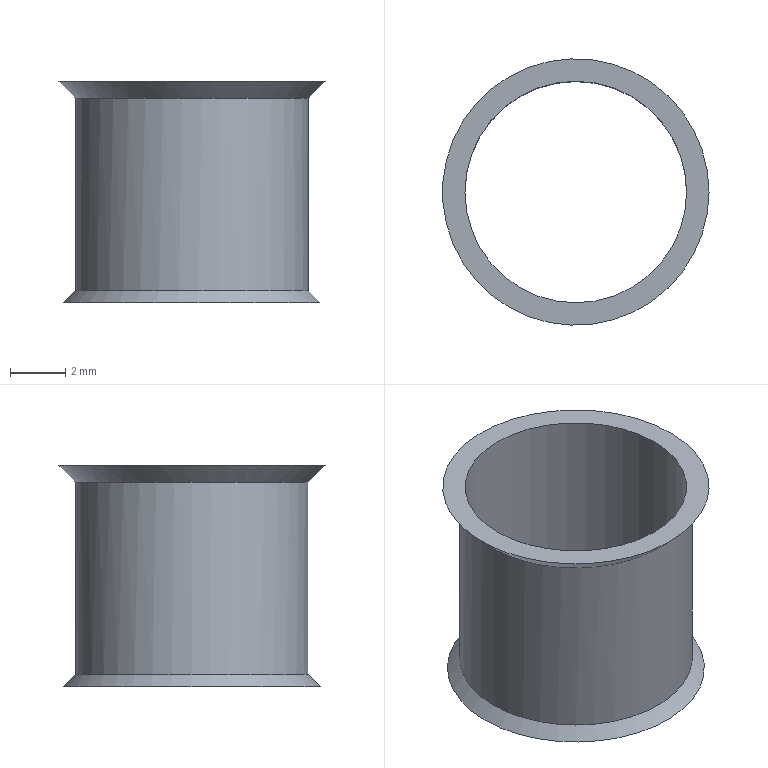Part | STEP file | 1 solid | 6 faces | box 9.62 x 9.62 x 8 mm | volume 49.009 mm3 | cylinder 2 | plane 2 | cone 2 | commonest cylinder face diameters 8 x1 8.4 x1
STEP:
#1=CARTESIAN_POINT('',(0.,0.,0.));
#2=DIRECTION('',(0.,0.,1.));
#3=DIRECTION('',(1.,0.,0.));
#4=AXIS2_PLACEMENT_3D('',#1,#2,#3);
#5=CARTESIAN_POINT('',(27.622,157.82,20.85));
#6=VERTEX_POINT('',#5);
#7=CARTESIAN_POINT('',(31.622,157.82,20.85));
#8=DIRECTION('',(0.,0.,1.));
#9=DIRECTION('',(-1.,0.,0.));
#10=AXIS2_PLACEMENT_3D('',#7,#8,#9);
#11=CIRCLE('',#10,4.);
#12=CARTESIAN_POINT('',(31.622,157.82,24.85));
#13=DIRECTION('',(0.,0.,-1.));
#14=DIRECTION('',(-1.,0.,0.));
#15=AXIS2_PLACEMENT_3D('',#12,#13,#14);
#16=CYLINDRICAL_SURFACE('',#15,4.);
#17=CARTESIAN_POINT('',(6.283,4.));
#18=DIRECTION('',(-1.,0.));
#19=VECTOR('',#18,1.);
#20=LINE('',#17,#19);
#21=(GEOMETRIC_REPRESENTATION_CONTEXT(2)PARAMETRIC_REPRESENTATION_CONTEXT()REPRESENTATION_CONTEXT('',''));
#22=DEFINITIONAL_REPRESENTATION('',(#20),#21);
#23=PCURVE('',#16,#22);
#24=CARTESIAN_POINT('',(39.122,157.82,20.85));
#25=DIRECTION('',(0.,0.,1.));
#26=DIRECTION('',(1.,0.,0.));
#27=AXIS2_PLACEMENT_3D('',#24,#25,#26);
#28=PLANE('',#27);
#29=CARTESIAN_POINT('',(-7.5,0.));
#30=DIRECTION('',(-1.,0.));
#31=AXIS2_PLACEMENT_2D('',#29,#30);
#32=CIRCLE('',#31,4.);
#33=(GEOMETRIC_REPRESENTATION_CONTEXT(2)PARAMETRIC_REPRESENTATION_CONTEXT()REPRESENTATION_CONTEXT('',''));
#34=DEFINITIONAL_REPRESENTATION('',(#32),#33);
#35=PCURVE('',#28,#34);
#36=SURFACE_CURVE('',#11,(#23,#35),.PCURVE_S1.);
#37=EDGE_CURVE('',#6,#6,#36,.T.);
#38=ORIENTED_EDGE('',*,*,#37,.T.);
#39=CARTESIAN_POINT('',(27.622,157.82,28.85));
#40=VERTEX_POINT('',#39);
#41=CARTESIAN_POINT('',(27.622,157.82,28.85));
#42=CARTESIAN_POINT('',(27.622,157.82,20.85));
#43=B_SPLINE_CURVE_WITH_KNOTS('',1,(#41,#42),.UNSPECIFIED.,.F.,.F.,(2,2),(-4.,4.),.PIECEWISE_BEZIER_KNOTS.);
#44=CARTESIAN_POINT('',(0.,0.));
#45=DIRECTION('',(0.,1.));
#46=VECTOR('',#45,1.);
#47=LINE('',#44,#46);
#48=(GEOMETRIC_REPRESENTATION_CONTEXT(2)PARAMETRIC_REPRESENTATION_CONTEXT()REPRESENTATION_CONTEXT('',''));
#49=DEFINITIONAL_REPRESENTATION('',(#47),#48);
#50=PCURVE('',#16,#49);
#51=CARTESIAN_POINT('',(6.283,0.));
#52=DIRECTION('',(0.,1.));
#53=VECTOR('',#52,1.);
#54=LINE('',#51,#53);
#55=(GEOMETRIC_REPRESENTATION_CONTEXT(2)PARAMETRIC_REPRESENTATION_CONTEXT()REPRESENTATION_CONTEXT('',''));
#56=DEFINITIONAL_REPRESENTATION('',(#54),#55);
#57=PCURVE('',#16,#56);
#58=SEAM_CURVE('',#43,(#50,#57),.PCURVE_S1.);
#59=EDGE_CURVE('',#40,#6,#58,.T.);
#60=ORIENTED_EDGE('',*,*,#59,.F.);
#61=CARTESIAN_POINT('',(31.622,157.82,28.85));
#62=DIRECTION('',(0.,0.,-1.));
#63=DIRECTION('',(-1.,0.,0.));
#64=AXIS2_PLACEMENT_3D('',#61,#62,#63);
#65=CIRCLE('',#64,4.);
#66=CARTESIAN_POINT('',(0.,-4.));
#67=DIRECTION('',(1.,0.));
#68=VECTOR('',#67,1.);
#69=LINE('',#66,#68);
#70=(GEOMETRIC_REPRESENTATION_CONTEXT(2)PARAMETRIC_REPRESENTATION_CONTEXT()REPRESENTATION_CONTEXT('',''));
#71=DEFINITIONAL_REPRESENTATION('',(#69),#70);
#72=PCURVE('',#16,#71);
#73=CARTESIAN_POINT('',(34.122,157.82,28.85));
#74=DIRECTION('',(0.,0.,-1.));
#75=DIRECTION('',(-1.,0.,0.));
#76=AXIS2_PLACEMENT_3D('',#73,#74,#75);
#77=PLANE('',#76);
#78=CARTESIAN_POINT('',(2.5,0.));
#79=DIRECTION('',(1.,0.));
#80=AXIS2_PLACEMENT_2D('',#78,#79);
#81=CIRCLE('',#80,4.);
#82=(GEOMETRIC_REPRESENTATION_CONTEXT(2)PARAMETRIC_REPRESENTATION_CONTEXT()REPRESENTATION_CONTEXT('',''));
#83=DEFINITIONAL_REPRESENTATION('',(#81),#82);
#84=PCURVE('',#77,#83);
#85=SURFACE_CURVE('',#65,(#72,#84),.PCURVE_S1.);
#86=EDGE_CURVE('',#40,#40,#85,.T.);
#87=ORIENTED_EDGE('',*,*,#86,.T.);
#88=ORIENTED_EDGE('',*,*,#59,.T.);
#89=EDGE_LOOP('',(#38,#60,#87,#88));
#90=FACE_BOUND('',#89,.F.);
#91=ADVANCED_FACE('',(#90),#16,.F.);
#92=ORIENTED_EDGE('',*,*,#86,.T.);
#93=EDGE_LOOP('',(#92));
#94=FACE_BOUND('',#93,.T.);
#95=CARTESIAN_POINT('',(36.432,157.82,28.85));
#96=VERTEX_POINT('',#95);
#97=CARTESIAN_POINT('',(31.622,157.82,28.85));
#98=DIRECTION('',(0.,0.,-1.));
#99=DIRECTION('',(1.,0.,0.));
#100=AXIS2_PLACEMENT_3D('',#97,#98,#99);
#101=CIRCLE('',#100,4.81);
#102=CARTESIAN_POINT('',(2.5,0.));
#103=DIRECTION('',(-1.,0.));
#104=AXIS2_PLACEMENT_2D('',#102,#103);
#105=CIRCLE('',#104,4.81);
#106=(GEOMETRIC_REPRESENTATION_CONTEXT(2)PARAMETRIC_REPRESENTATION_CONTEXT()REPRESENTATION_CONTEXT('',''));
#107=DEFINITIONAL_REPRESENTATION('',(#105),#106);
#108=PCURVE('',#77,#107);
#109=CARTESIAN_POINT('',(31.622,157.82,28.85));
#110=DIRECTION('',(0.,0.,1.));
#111=DIRECTION('',(1.,0.,0.));
#112=AXIS2_PLACEMENT_3D('',#109,#110,#111);
#113=CONICAL_SURFACE('',#112,4.81,0.7854);
#114=CARTESIAN_POINT('',(6.283,0.));
#115=DIRECTION('',(-1.,0.));
#116=VECTOR('',#115,1.);
#117=LINE('',#114,#116);
#118=(GEOMETRIC_REPRESENTATION_CONTEXT(2)PARAMETRIC_REPRESENTATION_CONTEXT()REPRESENTATION_CONTEXT('',''));
#119=DEFINITIONAL_REPRESENTATION('',(#117),#118);
#120=PCURVE('',#113,#119);
#121=SURFACE_CURVE('',#101,(#108,#120),.PCURVE_S1.);
#122=EDGE_CURVE('',#96,#96,#121,.T.);
#123=ORIENTED_EDGE('',*,*,#122,.F.);
#124=EDGE_LOOP('',(#123));
#125=FACE_BOUND('',#124,.T.);
#126=ADVANCED_FACE('',(#94,#125),#77,.F.);
#127=ORIENTED_EDGE('',*,*,#37,.T.);
#128=EDGE_LOOP('',(#127));
#129=FACE_BOUND('',#128,.T.);
#130=CARTESIAN_POINT('',(26.982,157.82,20.85));
#131=VERTEX_POINT('',#130);
#132=CARTESIAN_POINT('',(31.622,157.82,20.85));
#133=DIRECTION('',(0.,0.,1.));
#134=DIRECTION('',(-1.,0.,0.));
#135=AXIS2_PLACEMENT_3D('',#132,#133,#134);
#136=CIRCLE('',#135,4.64);
#137=CARTESIAN_POINT('',(-7.5,0.));
#138=DIRECTION('',(-1.,0.));
#139=AXIS2_PLACEMENT_2D('',#137,#138);
#140=CIRCLE('',#139,4.64);
#141=(GEOMETRIC_REPRESENTATION_CONTEXT(2)PARAMETRIC_REPRESENTATION_CONTEXT()REPRESENTATION_CONTEXT('',''));
#142=DEFINITIONAL_REPRESENTATION('',(#140),#141);
#143=PCURVE('',#28,#142);
#144=CARTESIAN_POINT('',(31.622,157.82,20.85));
#145=DIRECTION('',(0.,0.,-1.));
#146=DIRECTION('',(-1.,0.,0.));
#147=AXIS2_PLACEMENT_3D('',#144,#145,#146);
#148=CONICAL_SURFACE('',#147,4.64,0.7854);
#149=CARTESIAN_POINT('',(6.283,0.));
#150=DIRECTION('',(-1.,0.));
#151=VECTOR('',#150,1.);
#152=LINE('',#149,#151);
#153=(GEOMETRIC_REPRESENTATION_CONTEXT(2)PARAMETRIC_REPRESENTATION_CONTEXT()REPRESENTATION_CONTEXT('',''));
#154=DEFINITIONAL_REPRESENTATION('',(#152),#153);
#155=PCURVE('',#148,#154);
#156=SURFACE_CURVE('',#136,(#143,#155),.PCURVE_S1.);
#157=EDGE_CURVE('',#131,#131,#156,.T.);
#158=ORIENTED_EDGE('',*,*,#157,.F.);
#159=EDGE_LOOP('',(#158));
#160=FACE_BOUND('',#159,.T.);
#161=ADVANCED_FACE('',(#129,#160),#28,.F.);
#162=CARTESIAN_POINT('',(29.153,161.218,28.24));
#163=VERTEX_POINT('',#162);
#164=CARTESIAN_POINT('',(27.422,157.82,28.24));
#165=VERTEX_POINT('',#164);
#166=CARTESIAN_POINT('',(31.622,157.82,28.24));
#167=DIRECTION('',(0.,0.,1.));
#168=DIRECTION('',(-0.5878,0.809,0.));
#169=AXIS2_PLACEMENT_3D('',#166,#167,#168);
#170=CIRCLE('',#169,4.2);
#171=CARTESIAN_POINT('',(2.199,-0.61));
#172=DIRECTION('',(1.,0.));
#173=VECTOR('',#172,1.);
#174=LINE('',#171,#173);
#175=(GEOMETRIC_REPRESENTATION_CONTEXT(2)PARAMETRIC_REPRESENTATION_CONTEXT()REPRESENTATION_CONTEXT('',''));
#176=DEFINITIONAL_REPRESENTATION('',(#174),#175);
#177=PCURVE('',#113,#176);
#178=CARTESIAN_POINT('',(31.622,157.82,24.765));
#179=DIRECTION('',(0.,0.,-1.));
#180=DIRECTION('',(-1.,0.,0.));
#181=AXIS2_PLACEMENT_3D('',#178,#179,#180);
#182=CYLINDRICAL_SURFACE('',#181,4.2);
#183=CARTESIAN_POINT('',(0.9425,-3.475));
#184=DIRECTION('',(-1.,0.));
#185=VECTOR('',#184,1.);
#186=LINE('',#183,#185);
#187=(GEOMETRIC_REPRESENTATION_CONTEXT(2)PARAMETRIC_REPRESENTATION_CONTEXT()REPRESENTATION_CONTEXT('',''));
#188=DEFINITIONAL_REPRESENTATION('',(#186),#187);
#189=PCURVE('',#182,#188);
#190=SURFACE_CURVE('',#170,(#177,#189),.PCURVE_S1.);
#191=EDGE_CURVE('',#163,#165,#190,.T.);
#192=ORIENTED_EDGE('',*,*,#191,.T.);
#193=CARTESIAN_POINT('',(35.822,157.82,28.24));
#194=VERTEX_POINT('',#193);
#195=CARTESIAN_POINT('',(31.622,157.82,28.24));
#196=DIRECTION('',(0.,0.,1.));
#197=DIRECTION('',(-0.5878,0.809,0.));
#198=AXIS2_PLACEMENT_3D('',#195,#196,#197);
#199=CIRCLE('',#198,4.2);
#200=CARTESIAN_POINT('',(2.199,-0.61));
#201=DIRECTION('',(1.,0.));
#202=VECTOR('',#201,1.);
#203=LINE('',#200,#202);
#204=(GEOMETRIC_REPRESENTATION_CONTEXT(2)PARAMETRIC_REPRESENTATION_CONTEXT()REPRESENTATION_CONTEXT('',''));
#205=DEFINITIONAL_REPRESENTATION('',(#203),#204);
#206=PCURVE('',#113,#205);
#207=CARTESIAN_POINT('',(7.226,-3.475));
#208=DIRECTION('',(-1.,0.));
#209=VECTOR('',#208,1.);
#210=LINE('',#207,#209);
#211=(GEOMETRIC_REPRESENTATION_CONTEXT(2)PARAMETRIC_REPRESENTATION_CONTEXT()REPRESENTATION_CONTEXT('',''));
#212=DEFINITIONAL_REPRESENTATION('',(#210),#211);
#213=PCURVE('',#182,#212);
#214=SURFACE_CURVE('',#199,(#206,#213),.PCURVE_S1.);
#215=EDGE_CURVE('',#165,#194,#214,.T.);
#216=ORIENTED_EDGE('',*,*,#215,.T.);
#217=CARTESIAN_POINT('',(35.822,157.82,28.24));
#218=CARTESIAN_POINT('',(36.432,157.82,28.85));
#219=B_SPLINE_CURVE_WITH_KNOTS('',1,(#217,#218),.UNSPECIFIED.,.F.,.F.,(2,2),(-0.8627,0.),.PIECEWISE_BEZIER_KNOTS.);
#220=CARTESIAN_POINT('',(6.283,0.));
#221=DIRECTION('',(0.,1.));
#222=VECTOR('',#221,1.);
#223=LINE('',#220,#222);
#224=(GEOMETRIC_REPRESENTATION_CONTEXT(2)PARAMETRIC_REPRESENTATION_CONTEXT()REPRESENTATION_CONTEXT('',''));
#225=DEFINITIONAL_REPRESENTATION('',(#223),#224);
#226=PCURVE('',#113,#225);
#227=CARTESIAN_POINT('',(0.,0.));
#228=DIRECTION('',(0.,1.));
#229=VECTOR('',#228,1.);
#230=LINE('',#227,#229);
#231=(GEOMETRIC_REPRESENTATION_CONTEXT(2)PARAMETRIC_REPRESENTATION_CONTEXT()REPRESENTATION_CONTEXT('',''));
#232=DEFINITIONAL_REPRESENTATION('',(#230),#231);
#233=PCURVE('',#113,#232);
#234=SEAM_CURVE('',#219,(#226,#233),.PCURVE_S1.);
#235=EDGE_CURVE('',#194,#96,#234,.T.);
#236=ORIENTED_EDGE('',*,*,#235,.T.);
#237=ORIENTED_EDGE('',*,*,#122,.T.);
#238=ORIENTED_EDGE('',*,*,#235,.F.);
#239=CARTESIAN_POINT('',(31.622,157.82,28.24));
#240=DIRECTION('',(0.,0.,1.));
#241=DIRECTION('',(-0.5878,0.809,0.));
#242=AXIS2_PLACEMENT_3D('',#239,#240,#241);
#243=CIRCLE('',#242,4.2);
#244=CARTESIAN_POINT('',(-4.084,-0.61));
#245=DIRECTION('',(1.,0.));
#246=VECTOR('',#245,1.);
#247=LINE('',#244,#246);
#248=(GEOMETRIC_REPRESENTATION_CONTEXT(2)PARAMETRIC_REPRESENTATION_CONTEXT()REPRESENTATION_CONTEXT('',''));
#249=DEFINITIONAL_REPRESENTATION('',(#247),#248);
#250=PCURVE('',#113,#249);
#251=CARTESIAN_POINT('',(7.226,-3.475));
#252=DIRECTION('',(-1.,0.));
#253=VECTOR('',#252,1.);
#254=LINE('',#251,#253);
#255=(GEOMETRIC_REPRESENTATION_CONTEXT(2)PARAMETRIC_REPRESENTATION_CONTEXT()REPRESENTATION_CONTEXT('',''));
#256=DEFINITIONAL_REPRESENTATION('',(#254),#255);
#257=PCURVE('',#182,#256);
#258=SURFACE_CURVE('',#243,(#250,#257),.PCURVE_S1.);
#259=EDGE_CURVE('',#194,#163,#258,.T.);
#260=ORIENTED_EDGE('',*,*,#259,.T.);
#261=EDGE_LOOP('',(#192,#216,#236,#237,#238,#260));
#262=FACE_BOUND('',#261,.T.);
#263=ADVANCED_FACE('',(#262),#113,.T.);
#264=CARTESIAN_POINT('',(29.153,154.422,21.29));
#265=VERTEX_POINT('',#264);
#266=CARTESIAN_POINT('',(27.422,157.82,21.29));
#267=VERTEX_POINT('',#266);
#268=CARTESIAN_POINT('',(31.622,157.82,21.29));
#269=DIRECTION('',(0.,0.,-1.));
#270=DIRECTION('',(-0.5878,-0.809,0.));
#271=AXIS2_PLACEMENT_3D('',#268,#269,#270);
#272=CIRCLE('',#271,4.2);
#273=CARTESIAN_POINT('',(5.341,-0.44));
#274=DIRECTION('',(1.,0.));
#275=VECTOR('',#274,1.);
#276=LINE('',#273,#275);
#277=(GEOMETRIC_REPRESENTATION_CONTEXT(2)PARAMETRIC_REPRESENTATION_CONTEXT()REPRESENTATION_CONTEXT('',''));
#278=DEFINITIONAL_REPRESENTATION('',(#276),#277);
#279=PCURVE('',#148,#278);
#280=CARTESIAN_POINT('',(5.341,3.475));
#281=DIRECTION('',(1.,0.));
#282=VECTOR('',#281,1.);
#283=LINE('',#280,#282);
#284=(GEOMETRIC_REPRESENTATION_CONTEXT(2)PARAMETRIC_REPRESENTATION_CONTEXT()REPRESENTATION_CONTEXT('',''));
#285=DEFINITIONAL_REPRESENTATION('',(#283),#284);
#286=PCURVE('',#182,#285);
#287=SURFACE_CURVE('',#272,(#279,#286),.PCURVE_S1.);
#288=EDGE_CURVE('',#265,#267,#287,.T.);
#289=ORIENTED_EDGE('',*,*,#288,.T.);
#290=CARTESIAN_POINT('',(27.422,157.82,21.29));
#291=CARTESIAN_POINT('',(26.982,157.82,20.85));
#292=B_SPLINE_CURVE_WITH_KNOTS('',1,(#290,#291),.UNSPECIFIED.,.F.,.F.,(2,2),(-0.6223,0.),.PIECEWISE_BEZIER_KNOTS.);
#293=CARTESIAN_POINT('',(6.283,0.));
#294=DIRECTION('',(0.,1.));
#295=VECTOR('',#294,1.);
#296=LINE('',#293,#295);
#297=(GEOMETRIC_REPRESENTATION_CONTEXT(2)PARAMETRIC_REPRESENTATION_CONTEXT()REPRESENTATION_CONTEXT('',''));
#298=DEFINITIONAL_REPRESENTATION('',(#296),#297);
#299=PCURVE('',#148,#298);
#300=CARTESIAN_POINT('',(0.,0.));
#301=DIRECTION('',(0.,1.));
#302=VECTOR('',#301,1.);
#303=LINE('',#300,#302);
#304=(GEOMETRIC_REPRESENTATION_CONTEXT(2)PARAMETRIC_REPRESENTATION_CONTEXT()REPRESENTATION_CONTEXT('',''));
#305=DEFINITIONAL_REPRESENTATION('',(#303),#304);
#306=PCURVE('',#148,#305);
#307=SEAM_CURVE('',#292,(#299,#306),.PCURVE_S1.);
#308=EDGE_CURVE('',#267,#131,#307,.T.);
#309=ORIENTED_EDGE('',*,*,#308,.T.);
#310=ORIENTED_EDGE('',*,*,#157,.T.);
#311=ORIENTED_EDGE('',*,*,#308,.F.);
#312=CARTESIAN_POINT('',(31.622,157.82,21.29));
#313=DIRECTION('',(0.,0.,-1.));
#314=DIRECTION('',(-0.5878,-0.809,0.));
#315=AXIS2_PLACEMENT_3D('',#312,#313,#314);
#316=CIRCLE('',#315,4.2);
#317=CARTESIAN_POINT('',(-0.9425,-0.44));
#318=DIRECTION('',(1.,0.));
#319=VECTOR('',#318,1.);
#320=LINE('',#317,#319);
#321=(GEOMETRIC_REPRESENTATION_CONTEXT(2)PARAMETRIC_REPRESENTATION_CONTEXT()REPRESENTATION_CONTEXT('',''));
#322=DEFINITIONAL_REPRESENTATION('',(#320),#321);
#323=PCURVE('',#148,#322);
#324=CARTESIAN_POINT('',(-0.9425,3.475));
#325=DIRECTION('',(1.,0.));
#326=VECTOR('',#325,1.);
#327=LINE('',#324,#326);
#328=(GEOMETRIC_REPRESENTATION_CONTEXT(2)PARAMETRIC_REPRESENTATION_CONTEXT()REPRESENTATION_CONTEXT('',''));
#329=DEFINITIONAL_REPRESENTATION('',(#327),#328);
#330=PCURVE('',#182,#329);
#331=SURFACE_CURVE('',#316,(#323,#330),.PCURVE_S1.);
#332=EDGE_CURVE('',#267,#265,#331,.T.);
#333=ORIENTED_EDGE('',*,*,#332,.T.);
#334=EDGE_LOOP('',(#289,#309,#310,#311,#333));
#335=FACE_BOUND('',#334,.T.);
#336=ADVANCED_FACE('',(#335),#148,.T.);
#337=ORIENTED_EDGE('',*,*,#215,.F.);
#338=CARTESIAN_POINT('',(27.422,157.82,28.24));
#339=CARTESIAN_POINT('',(27.422,157.82,21.29));
#340=B_SPLINE_CURVE_WITH_KNOTS('',1,(#338,#339),.UNSPECIFIED.,.F.,.F.,(2,2),(-3.475,3.475),.PIECEWISE_BEZIER_KNOTS.);
#341=CARTESIAN_POINT('',(6.283,0.));
#342=DIRECTION('',(0.,1.));
#343=VECTOR('',#342,1.);
#344=LINE('',#341,#343);
#345=(GEOMETRIC_REPRESENTATION_CONTEXT(2)PARAMETRIC_REPRESENTATION_CONTEXT()REPRESENTATION_CONTEXT('',''));
#346=DEFINITIONAL_REPRESENTATION('',(#344),#345);
#347=PCURVE('',#182,#346);
#348=CARTESIAN_POINT('',(0.,0.));
#349=DIRECTION('',(0.,1.));
#350=VECTOR('',#349,1.);
#351=LINE('',#348,#350);
#352=(GEOMETRIC_REPRESENTATION_CONTEXT(2)PARAMETRIC_REPRESENTATION_CONTEXT()REPRESENTATION_CONTEXT('',''));
#353=DEFINITIONAL_REPRESENTATION('',(#351),#352);
#354=PCURVE('',#182,#353);
#355=SEAM_CURVE('',#340,(#347,#354),.PCURVE_S1.);
#356=EDGE_CURVE('',#165,#267,#355,.T.);
#357=ORIENTED_EDGE('',*,*,#356,.T.);
#358=ORIENTED_EDGE('',*,*,#288,.F.);
#359=ORIENTED_EDGE('',*,*,#332,.F.);
#360=ORIENTED_EDGE('',*,*,#356,.F.);
#361=ORIENTED_EDGE('',*,*,#191,.F.);
#362=ORIENTED_EDGE('',*,*,#259,.F.);
#363=EDGE_LOOP('',(#337,#357,#358,#359,#360,#361,#362));
#364=FACE_BOUND('',#363,.T.);
#365=ADVANCED_FACE('',(#364),#182,.T.);
#366=CLOSED_SHELL('',(#91,#126,#161,#263,#336,#365));
#367=MANIFOLD_SOLID_BREP('',#366);
#368=(LENGTH_UNIT()NAMED_UNIT(*)SI_UNIT(.MILLI.,.METRE.));
#369=UNCERTAINTY_MEASURE_WITH_UNIT(LENGTH_MEASURE(0.000005),#368,'','');
#370=(NAMED_UNIT(*)PLANE_ANGLE_UNIT()SI_UNIT($,.RADIAN.));
#371=(NAMED_UNIT(*)SI_UNIT($,.STERADIAN.)SOLID_ANGLE_UNIT());
#372=(GEOMETRIC_REPRESENTATION_CONTEXT(3)GLOBAL_UNCERTAINTY_ASSIGNED_CONTEXT((#369))GLOBAL_UNIT_ASSIGNED_CONTEXT((#368,#370,#371))REPRESENTATION_CONTEXT('',''));
#373=ADVANCED_BREP_SHAPE_REPRESENTATION('',(#4,#367),#372);